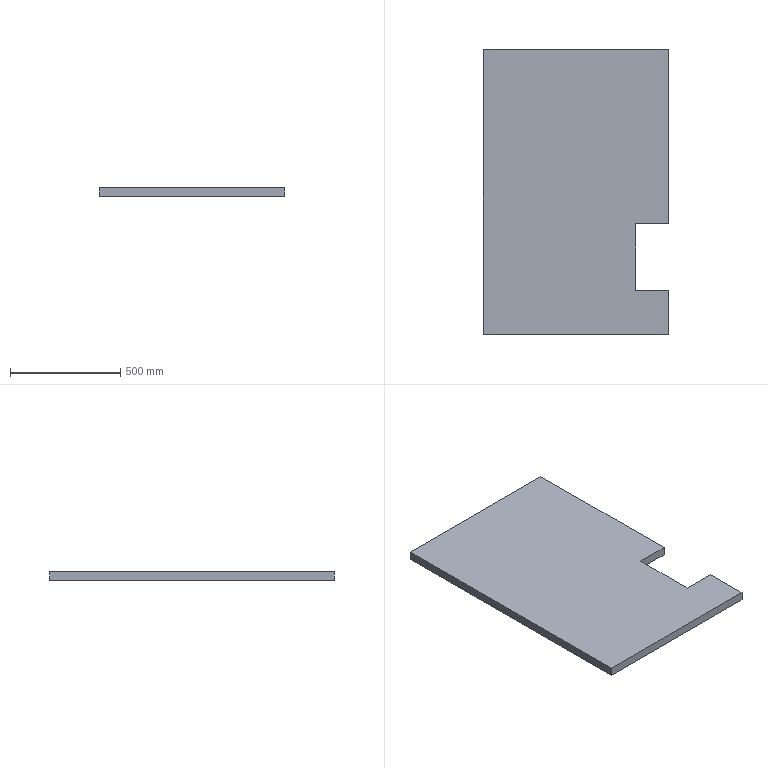Part | SolidWorks | features Extrusion 1 | 1 solid | 10 faces | box 840 x 1290 x 40 mm | volume 41544000 mm3 | plane 10
STEP:
#1=CARTESIAN_POINT('',(0.,1290.,0.));
#2=VERTEX_POINT('',#1);
#3=CARTESIAN_POINT('',(0.,0.,0.));
#4=VERTEX_POINT('',#3);
#5=CARTESIAN_POINT('',(0.,1290.,0.));
#6=DIRECTION('',(0.,-1.,0.));
#7=VECTOR('',#6,1000.);
#8=LINE('',#5,#7);
#9=EDGE_CURVE('',#2,#4,#8,.T.);
#10=ORIENTED_EDGE('',*,*,#9,.T.);
#11=CARTESIAN_POINT('',(0.,0.,40.));
#12=VERTEX_POINT('',#11);
#13=CARTESIAN_POINT('',(0.,0.,40.));
#14=DIRECTION('',(0.,0.,-1.));
#15=VECTOR('',#14,1000.);
#16=LINE('',#13,#15);
#17=EDGE_CURVE('',#12,#4,#16,.T.);
#18=ORIENTED_EDGE('',*,*,#17,.F.);
#19=CARTESIAN_POINT('',(0.,1290.,40.));
#20=VERTEX_POINT('',#19);
#21=CARTESIAN_POINT('',(0.,1290.,40.));
#22=DIRECTION('',(0.,-1.,0.));
#23=VECTOR('',#22,1000.);
#24=LINE('',#21,#23);
#25=EDGE_CURVE('',#20,#12,#24,.T.);
#26=ORIENTED_EDGE('',*,*,#25,.F.);
#27=CARTESIAN_POINT('',(0.,1290.,40.));
#28=DIRECTION('',(0.,0.,-1.));
#29=VECTOR('',#28,1000.);
#30=LINE('',#27,#29);
#31=EDGE_CURVE('',#20,#2,#30,.T.);
#32=ORIENTED_EDGE('',*,*,#31,.T.);
#33=EDGE_LOOP('',(#10,#18,#26,#32));
#34=FACE_OUTER_BOUND('',#33,.T.);
#35=CARTESIAN_POINT('',(0.,1290.,40.));
#36=DIRECTION('',(1.,0.,0.));
#37=DIRECTION('',(0.,0.,-1.));
#38=AXIS2_PLACEMENT_3D('',#35,#36,#37);
#39=PLANE('',#38);
#40=ADVANCED_FACE('',(#34),#39,.F.);
#41=CARTESIAN_POINT('',(840.,0.,0.));
#42=VERTEX_POINT('',#41);
#43=CARTESIAN_POINT('',(0.,0.,0.));
#44=DIRECTION('',(1.,0.,0.));
#45=VECTOR('',#44,1000.);
#46=LINE('',#43,#45);
#47=EDGE_CURVE('',#4,#42,#46,.T.);
#48=ORIENTED_EDGE('',*,*,#47,.T.);
#49=CARTESIAN_POINT('',(840.,0.,40.));
#50=VERTEX_POINT('',#49);
#51=CARTESIAN_POINT('',(840.,0.,40.));
#52=DIRECTION('',(0.,0.,-1.));
#53=VECTOR('',#52,1000.);
#54=LINE('',#51,#53);
#55=EDGE_CURVE('',#50,#42,#54,.T.);
#56=ORIENTED_EDGE('',*,*,#55,.F.);
#57=CARTESIAN_POINT('',(0.,0.,40.));
#58=DIRECTION('',(1.,0.,0.));
#59=VECTOR('',#58,1000.);
#60=LINE('',#57,#59);
#61=EDGE_CURVE('',#12,#50,#60,.T.);
#62=ORIENTED_EDGE('',*,*,#61,.F.);
#63=ORIENTED_EDGE('',*,*,#17,.T.);
#64=EDGE_LOOP('',(#48,#56,#62,#63));
#65=FACE_OUTER_BOUND('',#64,.T.);
#66=CARTESIAN_POINT('',(0.,0.,40.));
#67=DIRECTION('',(0.,1.,0.));
#68=DIRECTION('',(0.,0.,1.));
#69=AXIS2_PLACEMENT_3D('',#66,#67,#68);
#70=PLANE('',#69);
#71=ADVANCED_FACE('',(#65),#70,.F.);
#72=CARTESIAN_POINT('',(840.,200.,0.));
#73=VERTEX_POINT('',#72);
#74=CARTESIAN_POINT('',(840.,200.,0.));
#75=DIRECTION('',(0.,1.,0.));
#76=VECTOR('',#75,1000.);
#77=LINE('',#74,#76);
#78=EDGE_CURVE('',#42,#73,#77,.T.);
#79=ORIENTED_EDGE('',*,*,#78,.T.);
#80=CARTESIAN_POINT('',(840.,200.,40.));
#81=VERTEX_POINT('',#80);
#82=CARTESIAN_POINT('',(840.,200.,40.));
#83=DIRECTION('',(0.,0.,-1.));
#84=VECTOR('',#83,1000.);
#85=LINE('',#82,#84);
#86=EDGE_CURVE('',#81,#73,#85,.T.);
#87=ORIENTED_EDGE('',*,*,#86,.F.);
#88=CARTESIAN_POINT('',(840.,200.,40.));
#89=DIRECTION('',(0.,1.,0.));
#90=VECTOR('',#89,1000.);
#91=LINE('',#88,#90);
#92=EDGE_CURVE('',#50,#81,#91,.T.);
#93=ORIENTED_EDGE('',*,*,#92,.F.);
#94=ORIENTED_EDGE('',*,*,#55,.T.);
#95=EDGE_LOOP('',(#79,#87,#93,#94));
#96=FACE_OUTER_BOUND('',#95,.T.);
#97=CARTESIAN_POINT('',(840.,200.,40.));
#98=DIRECTION('',(-1.,0.,0.));
#99=DIRECTION('',(0.,0.,1.));
#100=AXIS2_PLACEMENT_3D('',#97,#98,#99);
#101=PLANE('',#100);
#102=ADVANCED_FACE('',(#96),#101,.F.);
#103=CARTESIAN_POINT('',(690.,200.,0.));
#104=VERTEX_POINT('',#103);
#105=CARTESIAN_POINT('',(690.,200.,0.));
#106=DIRECTION('',(-1.,0.,0.));
#107=VECTOR('',#106,1000.);
#108=LINE('',#105,#107);
#109=EDGE_CURVE('',#73,#104,#108,.T.);
#110=ORIENTED_EDGE('',*,*,#109,.T.);
#111=CARTESIAN_POINT('',(690.,200.,40.));
#112=VERTEX_POINT('',#111);
#113=CARTESIAN_POINT('',(690.,200.,40.));
#114=DIRECTION('',(0.,0.,-1.));
#115=VECTOR('',#114,1000.);
#116=LINE('',#113,#115);
#117=EDGE_CURVE('',#112,#104,#116,.T.);
#118=ORIENTED_EDGE('',*,*,#117,.F.);
#119=CARTESIAN_POINT('',(690.,200.,40.));
#120=DIRECTION('',(-1.,0.,0.));
#121=VECTOR('',#120,1000.);
#122=LINE('',#119,#121);
#123=EDGE_CURVE('',#81,#112,#122,.T.);
#124=ORIENTED_EDGE('',*,*,#123,.F.);
#125=ORIENTED_EDGE('',*,*,#86,.T.);
#126=EDGE_LOOP('',(#110,#118,#124,#125));
#127=FACE_OUTER_BOUND('',#126,.T.);
#128=CARTESIAN_POINT('',(690.,200.,40.));
#129=DIRECTION('',(0.,-1.,0.));
#130=DIRECTION('',(0.,0.,-1.));
#131=AXIS2_PLACEMENT_3D('',#128,#129,#130);
#132=PLANE('',#131);
#133=ADVANCED_FACE('',(#127),#132,.F.);
#134=CARTESIAN_POINT('',(690.,500.,0.));
#135=VERTEX_POINT('',#134);
#136=CARTESIAN_POINT('',(690.,200.,0.));
#137=DIRECTION('',(0.,1.,0.));
#138=VECTOR('',#137,1000.);
#139=LINE('',#136,#138);
#140=EDGE_CURVE('',#104,#135,#139,.T.);
#141=ORIENTED_EDGE('',*,*,#140,.T.);
#142=CARTESIAN_POINT('',(690.,500.,40.));
#143=VERTEX_POINT('',#142);
#144=CARTESIAN_POINT('',(690.,500.,40.));
#145=DIRECTION('',(0.,0.,-1.));
#146=VECTOR('',#145,1000.);
#147=LINE('',#144,#146);
#148=EDGE_CURVE('',#143,#135,#147,.T.);
#149=ORIENTED_EDGE('',*,*,#148,.F.);
#150=CARTESIAN_POINT('',(690.,200.,40.));
#151=DIRECTION('',(0.,1.,0.));
#152=VECTOR('',#151,1000.);
#153=LINE('',#150,#152);
#154=EDGE_CURVE('',#112,#143,#153,.T.);
#155=ORIENTED_EDGE('',*,*,#154,.F.);
#156=ORIENTED_EDGE('',*,*,#117,.T.);
#157=EDGE_LOOP('',(#141,#149,#155,#156));
#158=FACE_OUTER_BOUND('',#157,.T.);
#159=CARTESIAN_POINT('',(690.,200.,40.));
#160=DIRECTION('',(-1.,0.,0.));
#161=DIRECTION('',(0.,0.,1.));
#162=AXIS2_PLACEMENT_3D('',#159,#160,#161);
#163=PLANE('',#162);
#164=ADVANCED_FACE('',(#158),#163,.F.);
#165=CARTESIAN_POINT('',(840.,500.,0.));
#166=VERTEX_POINT('',#165);
#167=CARTESIAN_POINT('',(690.,500.,0.));
#168=DIRECTION('',(1.,0.,0.));
#169=VECTOR('',#168,1000.);
#170=LINE('',#167,#169);
#171=EDGE_CURVE('',#135,#166,#170,.T.);
#172=ORIENTED_EDGE('',*,*,#171,.T.);
#173=CARTESIAN_POINT('',(840.,500.,40.));
#174=VERTEX_POINT('',#173);
#175=CARTESIAN_POINT('',(840.,500.,40.));
#176=DIRECTION('',(0.,0.,-1.));
#177=VECTOR('',#176,1000.);
#178=LINE('',#175,#177);
#179=EDGE_CURVE('',#174,#166,#178,.T.);
#180=ORIENTED_EDGE('',*,*,#179,.F.);
#181=CARTESIAN_POINT('',(690.,500.,40.));
#182=DIRECTION('',(1.,0.,0.));
#183=VECTOR('',#182,1000.);
#184=LINE('',#181,#183);
#185=EDGE_CURVE('',#143,#174,#184,.T.);
#186=ORIENTED_EDGE('',*,*,#185,.F.);
#187=ORIENTED_EDGE('',*,*,#148,.T.);
#188=EDGE_LOOP('',(#172,#180,#186,#187));
#189=FACE_OUTER_BOUND('',#188,.T.);
#190=CARTESIAN_POINT('',(690.,500.,40.));
#191=DIRECTION('',(0.,1.,0.));
#192=DIRECTION('',(0.,0.,1.));
#193=AXIS2_PLACEMENT_3D('',#190,#191,#192);
#194=PLANE('',#193);
#195=ADVANCED_FACE('',(#189),#194,.F.);
#196=CARTESIAN_POINT('',(840.,1290.,0.));
#197=VERTEX_POINT('',#196);
#198=CARTESIAN_POINT('',(840.,500.,0.));
#199=DIRECTION('',(0.,1.,0.));
#200=VECTOR('',#199,1000.);
#201=LINE('',#198,#200);
#202=EDGE_CURVE('',#166,#197,#201,.T.);
#203=ORIENTED_EDGE('',*,*,#202,.T.);
#204=CARTESIAN_POINT('',(840.,1290.,40.));
#205=VERTEX_POINT('',#204);
#206=CARTESIAN_POINT('',(840.,1290.,40.));
#207=DIRECTION('',(0.,0.,-1.));
#208=VECTOR('',#207,1000.);
#209=LINE('',#206,#208);
#210=EDGE_CURVE('',#205,#197,#209,.T.);
#211=ORIENTED_EDGE('',*,*,#210,.F.);
#212=CARTESIAN_POINT('',(840.,500.,40.));
#213=DIRECTION('',(0.,1.,0.));
#214=VECTOR('',#213,1000.);
#215=LINE('',#212,#214);
#216=EDGE_CURVE('',#174,#205,#215,.T.);
#217=ORIENTED_EDGE('',*,*,#216,.F.);
#218=ORIENTED_EDGE('',*,*,#179,.T.);
#219=EDGE_LOOP('',(#203,#211,#217,#218));
#220=FACE_OUTER_BOUND('',#219,.T.);
#221=CARTESIAN_POINT('',(840.,500.,40.));
#222=DIRECTION('',(-1.,0.,0.));
#223=DIRECTION('',(0.,0.,1.));
#224=AXIS2_PLACEMENT_3D('',#221,#222,#223);
#225=PLANE('',#224);
#226=ADVANCED_FACE('',(#220),#225,.F.);
#227=CARTESIAN_POINT('',(840.,1290.,0.));
#228=DIRECTION('',(-1.,0.,0.));
#229=VECTOR('',#228,1000.);
#230=LINE('',#227,#229);
#231=EDGE_CURVE('',#197,#2,#230,.T.);
#232=ORIENTED_EDGE('',*,*,#231,.T.);
#233=ORIENTED_EDGE('',*,*,#31,.F.);
#234=CARTESIAN_POINT('',(840.,1290.,40.));
#235=DIRECTION('',(-1.,0.,0.));
#236=VECTOR('',#235,1000.);
#237=LINE('',#234,#236);
#238=EDGE_CURVE('',#205,#20,#237,.T.);
#239=ORIENTED_EDGE('',*,*,#238,.F.);
#240=ORIENTED_EDGE('',*,*,#210,.T.);
#241=EDGE_LOOP('',(#232,#233,#239,#240));
#242=FACE_OUTER_BOUND('',#241,.T.);
#243=CARTESIAN_POINT('',(840.,1290.,40.));
#244=DIRECTION('',(0.,-1.,0.));
#245=DIRECTION('',(0.,0.,-1.));
#246=AXIS2_PLACEMENT_3D('',#243,#244,#245);
#247=PLANE('',#246);
#248=ADVANCED_FACE('',(#242),#247,.F.);
#249=ORIENTED_EDGE('',*,*,#25,.T.);
#250=ORIENTED_EDGE('',*,*,#61,.T.);
#251=ORIENTED_EDGE('',*,*,#92,.T.);
#252=ORIENTED_EDGE('',*,*,#123,.T.);
#253=ORIENTED_EDGE('',*,*,#154,.T.);
#254=ORIENTED_EDGE('',*,*,#185,.T.);
#255=ORIENTED_EDGE('',*,*,#216,.T.);
#256=ORIENTED_EDGE('',*,*,#238,.T.);
#257=EDGE_LOOP('',(#249,#250,#251,#252,#253,#254,#255,#256));
#258=FACE_OUTER_BOUND('',#257,.T.);
#259=CARTESIAN_POINT('',(0.,0.,40.));
#260=DIRECTION('',(0.,0.,1.));
#261=DIRECTION('',(1.,0.,0.));
#262=AXIS2_PLACEMENT_3D('',#259,#260,#261);
#263=PLANE('',#262);
#264=ADVANCED_FACE('',(#258),#263,.T.);
#265=ORIENTED_EDGE('',*,*,#9,.F.);
#266=ORIENTED_EDGE('',*,*,#231,.F.);
#267=ORIENTED_EDGE('',*,*,#202,.F.);
#268=ORIENTED_EDGE('',*,*,#171,.F.);
#269=ORIENTED_EDGE('',*,*,#140,.F.);
#270=ORIENTED_EDGE('',*,*,#109,.F.);
#271=ORIENTED_EDGE('',*,*,#78,.F.);
#272=ORIENTED_EDGE('',*,*,#47,.F.);
#273=EDGE_LOOP('',(#265,#266,#267,#268,#269,#270,#271,#272));
#274=FACE_OUTER_BOUND('',#273,.T.);
#275=CARTESIAN_POINT('',(0.,0.,0.));
#276=DIRECTION('',(0.,0.,1.));
#277=DIRECTION('',(1.,0.,0.));
#278=AXIS2_PLACEMENT_3D('',#275,#276,#277);
#279=PLANE('',#278);
#280=ADVANCED_FACE('',(#274),#279,.F.);
#281=CLOSED_SHELL('',(#40,#71,#102,#133,#164,#195,#226,#248,#264,#280));
#282=MANIFOLD_SOLID_BREP('',#281);
#283=CARTESIAN_POINT('',(0.,0.,0.));
#284=DIRECTION('',(0.,0.,1.));
#285=DIRECTION('',(1.,0.,0.));
#286=AXIS2_PLACEMENT_3D('',#283,#284,#285);
#287=(LENGTH_UNIT()NAMED_UNIT(*)SI_UNIT(.MILLI.,.METRE.));
#288=UNCERTAINTY_MEASURE_WITH_UNIT(LENGTH_MEASURE(0.00001),#287,'','');
#289=(NAMED_UNIT(*)PLANE_ANGLE_UNIT()SI_UNIT($,.RADIAN.));
#290=(NAMED_UNIT(*)SI_UNIT($,.STERADIAN.)SOLID_ANGLE_UNIT());
#291=(GEOMETRIC_REPRESENTATION_CONTEXT(3)GLOBAL_UNCERTAINTY_ASSIGNED_CONTEXT((#288))GLOBAL_UNIT_ASSIGNED_CONTEXT((#287,#289,#290))REPRESENTATION_CONTEXT('',''));
#292=ADVANCED_BREP_SHAPE_REPRESENTATION('',(#282,#286),#291);